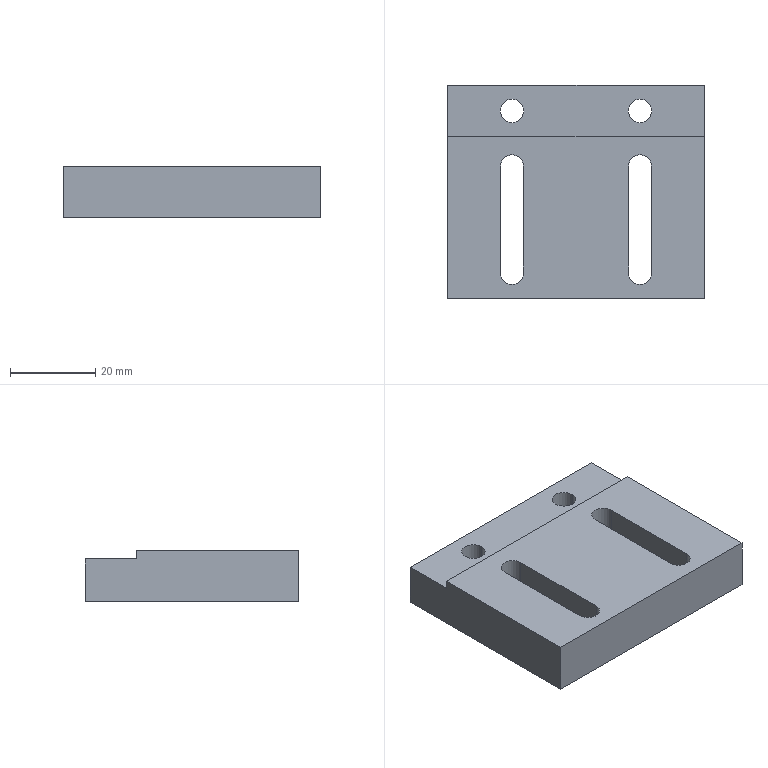Part | SolidWorks | features Cut 1, Extrusion 1, HoleWzd 1, ICE 1 | 1 solid | 26 faces | box 60 x 50 x 12 mm | volume 29704 mm3 | plane 14 | cylinder 12 | commonest cylinder face diameters 5.4 x4 5.5 x4 10 x4
STEP:
#1=CARTESIAN_POINT('',(20.,19.,-0.6));
#2=VERTEX_POINT('',#1);
#3=CARTESIAN_POINT('',(10.,19.,-0.6));
#4=VERTEX_POINT('',#3);
#5=CARTESIAN_POINT('',(15.,19.,-0.6));
#6=DIRECTION('',(0.,0.,-1.));
#7=DIRECTION('',(-1.,0.,0.));
#8=AXIS2_PLACEMENT_3D('',#5,#6,#7);
#9=CIRCLE('',#8,5.);
#10=EDGE_CURVE('',#2,#4,#9,.T.);
#11=ORIENTED_EDGE('',*,*,#10,.F.);
#12=CARTESIAN_POINT('',(20.,19.,-6.));
#13=VERTEX_POINT('',#12);
#14=CARTESIAN_POINT('',(20.,19.,-6.));
#15=DIRECTION('',(0.,0.,-1.));
#16=VECTOR('',#15,1000.);
#17=LINE('',#14,#16);
#18=EDGE_CURVE('',#2,#13,#17,.T.);
#19=ORIENTED_EDGE('',*,*,#18,.T.);
#20=CARTESIAN_POINT('',(10.,19.,-6.));
#21=VERTEX_POINT('',#20);
#22=CARTESIAN_POINT('',(15.,19.,-6.));
#23=DIRECTION('',(0.,0.,-1.));
#24=DIRECTION('',(-1.,0.,0.));
#25=AXIS2_PLACEMENT_3D('',#22,#23,#24);
#26=CIRCLE('',#25,5.);
#27=EDGE_CURVE('',#13,#21,#26,.T.);
#28=ORIENTED_EDGE('',*,*,#27,.T.);
#29=CARTESIAN_POINT('',(10.,19.,-6.));
#30=DIRECTION('',(0.,0.,-1.));
#31=VECTOR('',#30,1000.);
#32=LINE('',#29,#31);
#33=EDGE_CURVE('',#4,#21,#32,.T.);
#34=ORIENTED_EDGE('',*,*,#33,.F.);
#35=EDGE_LOOP('',(#11,#19,#28,#34));
#36=FACE_OUTER_BOUND('',#35,.T.);
#37=CARTESIAN_POINT('',(15.,19.,-6.));
#38=DIRECTION('',(0.,0.,-1.));
#39=DIRECTION('',(-1.,0.,0.));
#40=AXIS2_PLACEMENT_3D('',#37,#38,#39);
#41=CYLINDRICAL_SURFACE('',#40,5.);
#42=ADVANCED_FACE('',(#36),#41,.F.);
#43=CARTESIAN_POINT('',(12.25,19.,4.));
#44=VERTEX_POINT('',#43);
#45=CARTESIAN_POINT('',(17.75,19.,4.));
#46=VERTEX_POINT('',#45);
#47=CARTESIAN_POINT('',(15.,19.,4.));
#48=DIRECTION('',(0.,0.,1.));
#49=DIRECTION('',(1.,0.,0.));
#50=AXIS2_PLACEMENT_3D('',#47,#48,#49);
#51=CIRCLE('',#50,2.75);
#52=EDGE_CURVE('',#44,#46,#51,.T.);
#53=ORIENTED_EDGE('',*,*,#52,.T.);
#54=CARTESIAN_POINT('',(17.75,19.,-0.6));
#55=VERTEX_POINT('',#54);
#56=CARTESIAN_POINT('',(17.75,19.,-6.));
#57=DIRECTION('',(0.,0.,-1.));
#58=VECTOR('',#57,1000.);
#59=LINE('',#56,#58);
#60=EDGE_CURVE('',#46,#55,#59,.T.);
#61=ORIENTED_EDGE('',*,*,#60,.T.);
#62=CARTESIAN_POINT('',(12.25,19.,-0.6));
#63=VERTEX_POINT('',#62);
#64=CARTESIAN_POINT('',(15.,19.,-0.6));
#65=DIRECTION('',(0.,0.,-1.));
#66=DIRECTION('',(-1.,0.,0.));
#67=AXIS2_PLACEMENT_3D('',#64,#65,#66);
#68=CIRCLE('',#67,2.75);
#69=EDGE_CURVE('',#55,#63,#68,.T.);
#70=ORIENTED_EDGE('',*,*,#69,.T.);
#71=CARTESIAN_POINT('',(12.25,19.,-6.));
#72=DIRECTION('',(0.,0.,-1.));
#73=VECTOR('',#72,1000.);
#74=LINE('',#71,#73);
#75=EDGE_CURVE('',#44,#63,#74,.T.);
#76=ORIENTED_EDGE('',*,*,#75,.F.);
#77=EDGE_LOOP('',(#53,#61,#70,#76));
#78=FACE_OUTER_BOUND('',#77,.T.);
#79=CARTESIAN_POINT('',(15.,19.,-6.));
#80=DIRECTION('',(0.,0.,-1.));
#81=DIRECTION('',(-1.,0.,0.));
#82=AXIS2_PLACEMENT_3D('',#79,#80,#81);
#83=CYLINDRICAL_SURFACE('',#82,2.75);
#84=ADVANCED_FACE('',(#78),#83,.F.);
#85=CARTESIAN_POINT('',(-10.,19.,-0.6));
#86=VERTEX_POINT('',#85);
#87=CARTESIAN_POINT('',(-20.,19.,-0.6));
#88=VERTEX_POINT('',#87);
#89=CARTESIAN_POINT('',(-15.,19.,-0.6));
#90=DIRECTION('',(0.,0.,-1.));
#91=DIRECTION('',(-1.,0.,0.));
#92=AXIS2_PLACEMENT_3D('',#89,#90,#91);
#93=CIRCLE('',#92,5.);
#94=EDGE_CURVE('',#86,#88,#93,.T.);
#95=ORIENTED_EDGE('',*,*,#94,.F.);
#96=CARTESIAN_POINT('',(-10.,19.,-6.));
#97=VERTEX_POINT('',#96);
#98=CARTESIAN_POINT('',(-10.,19.,-6.));
#99=DIRECTION('',(0.,0.,-1.));
#100=VECTOR('',#99,1000.);
#101=LINE('',#98,#100);
#102=EDGE_CURVE('',#86,#97,#101,.T.);
#103=ORIENTED_EDGE('',*,*,#102,.T.);
#104=CARTESIAN_POINT('',(-20.,19.,-6.));
#105=VERTEX_POINT('',#104);
#106=CARTESIAN_POINT('',(-15.,19.,-6.));
#107=DIRECTION('',(0.,0.,-1.));
#108=DIRECTION('',(-1.,0.,0.));
#109=AXIS2_PLACEMENT_3D('',#106,#107,#108);
#110=CIRCLE('',#109,5.);
#111=EDGE_CURVE('',#97,#105,#110,.T.);
#112=ORIENTED_EDGE('',*,*,#111,.T.);
#113=CARTESIAN_POINT('',(-20.,19.,-6.));
#114=DIRECTION('',(0.,0.,-1.));
#115=VECTOR('',#114,1000.);
#116=LINE('',#113,#115);
#117=EDGE_CURVE('',#88,#105,#116,.T.);
#118=ORIENTED_EDGE('',*,*,#117,.F.);
#119=EDGE_LOOP('',(#95,#103,#112,#118));
#120=FACE_OUTER_BOUND('',#119,.T.);
#121=CARTESIAN_POINT('',(-15.,19.,-6.));
#122=DIRECTION('',(0.,0.,-1.));
#123=DIRECTION('',(-1.,0.,0.));
#124=AXIS2_PLACEMENT_3D('',#121,#122,#123);
#125=CYLINDRICAL_SURFACE('',#124,5.);
#126=ADVANCED_FACE('',(#120),#125,.F.);
#127=CARTESIAN_POINT('',(-17.75,19.,4.));
#128=VERTEX_POINT('',#127);
#129=CARTESIAN_POINT('',(-12.25,19.,4.));
#130=VERTEX_POINT('',#129);
#131=CARTESIAN_POINT('',(-15.,19.,4.));
#132=DIRECTION('',(0.,0.,1.));
#133=DIRECTION('',(1.,0.,0.));
#134=AXIS2_PLACEMENT_3D('',#131,#132,#133);
#135=CIRCLE('',#134,2.75);
#136=EDGE_CURVE('',#128,#130,#135,.T.);
#137=ORIENTED_EDGE('',*,*,#136,.T.);
#138=CARTESIAN_POINT('',(-12.25,19.,-0.6));
#139=VERTEX_POINT('',#138);
#140=CARTESIAN_POINT('',(-12.25,19.,-6.));
#141=DIRECTION('',(0.,0.,-1.));
#142=VECTOR('',#141,1000.);
#143=LINE('',#140,#142);
#144=EDGE_CURVE('',#130,#139,#143,.T.);
#145=ORIENTED_EDGE('',*,*,#144,.T.);
#146=CARTESIAN_POINT('',(-17.75,19.,-0.6));
#147=VERTEX_POINT('',#146);
#148=CARTESIAN_POINT('',(-15.,19.,-0.6));
#149=DIRECTION('',(0.,0.,-1.));
#150=DIRECTION('',(-1.,0.,0.));
#151=AXIS2_PLACEMENT_3D('',#148,#149,#150);
#152=CIRCLE('',#151,2.75);
#153=EDGE_CURVE('',#139,#147,#152,.T.);
#154=ORIENTED_EDGE('',*,*,#153,.T.);
#155=CARTESIAN_POINT('',(-17.75,19.,-6.));
#156=DIRECTION('',(0.,0.,-1.));
#157=VECTOR('',#156,1000.);
#158=LINE('',#155,#157);
#159=EDGE_CURVE('',#128,#147,#158,.T.);
#160=ORIENTED_EDGE('',*,*,#159,.F.);
#161=EDGE_LOOP('',(#137,#145,#154,#160));
#162=FACE_OUTER_BOUND('',#161,.T.);
#163=CARTESIAN_POINT('',(-15.,19.,-6.));
#164=DIRECTION('',(0.,0.,-1.));
#165=DIRECTION('',(-1.,0.,0.));
#166=AXIS2_PLACEMENT_3D('',#163,#164,#165);
#167=CYLINDRICAL_SURFACE('',#166,2.75);
#168=ADVANCED_FACE('',(#162),#167,.F.);
#169=CARTESIAN_POINT('',(30.,25.,4.));
#170=VERTEX_POINT('',#169);
#171=CARTESIAN_POINT('',(-30.,25.,4.));
#172=VERTEX_POINT('',#171);
#173=CARTESIAN_POINT('',(-30.,25.,4.));
#174=DIRECTION('',(-1.,0.,0.));
#175=VECTOR('',#174,1000.);
#176=LINE('',#173,#175);
#177=EDGE_CURVE('',#170,#172,#176,.T.);
#178=ORIENTED_EDGE('',*,*,#177,.F.);
#179=CARTESIAN_POINT('',(30.,25.,-6.));
#180=VERTEX_POINT('',#179);
#181=CARTESIAN_POINT('',(30.,25.,6.));
#182=DIRECTION('',(0.,0.,-1.));
#183=VECTOR('',#182,1000.);
#184=LINE('',#181,#183);
#185=EDGE_CURVE('',#170,#180,#184,.T.);
#186=ORIENTED_EDGE('',*,*,#185,.T.);
#187=CARTESIAN_POINT('',(-30.,25.,-6.));
#188=VERTEX_POINT('',#187);
#189=CARTESIAN_POINT('',(-30.,25.,-6.));
#190=DIRECTION('',(-1.,0.,0.));
#191=VECTOR('',#190,1000.);
#192=LINE('',#189,#191);
#193=EDGE_CURVE('',#180,#188,#192,.T.);
#194=ORIENTED_EDGE('',*,*,#193,.T.);
#195=CARTESIAN_POINT('',(-30.,25.,6.));
#196=DIRECTION('',(0.,0.,-1.));
#197=VECTOR('',#196,1000.);
#198=LINE('',#195,#197);
#199=EDGE_CURVE('',#172,#188,#198,.T.);
#200=ORIENTED_EDGE('',*,*,#199,.F.);
#201=EDGE_LOOP('',(#178,#186,#194,#200));
#202=FACE_OUTER_BOUND('',#201,.T.);
#203=CARTESIAN_POINT('',(-30.,25.,6.));
#204=DIRECTION('',(0.,-1.,0.));
#205=DIRECTION('',(0.,0.,-1.));
#206=AXIS2_PLACEMENT_3D('',#203,#204,#205);
#207=PLANE('',#206);
#208=ADVANCED_FACE('',(#202),#207,.F.);
#209=CARTESIAN_POINT('',(30.,13.,4.));
#210=VERTEX_POINT('',#209);
#211=CARTESIAN_POINT('',(30.,25.,4.));
#212=DIRECTION('',(0.,1.,0.));
#213=VECTOR('',#212,1000.);
#214=LINE('',#211,#213);
#215=EDGE_CURVE('',#210,#170,#214,.T.);
#216=ORIENTED_EDGE('',*,*,#215,.F.);
#217=CARTESIAN_POINT('',(30.,13.,6.));
#218=VERTEX_POINT('',#217);
#219=CARTESIAN_POINT('',(30.,13.,4.));
#220=DIRECTION('',(0.,0.,1.));
#221=VECTOR('',#220,1000.);
#222=LINE('',#219,#221);
#223=EDGE_CURVE('',#210,#218,#222,.T.);
#224=ORIENTED_EDGE('',*,*,#223,.T.);
#225=CARTESIAN_POINT('',(30.,-25.,6.));
#226=VERTEX_POINT('',#225);
#227=CARTESIAN_POINT('',(30.,25.,6.));
#228=DIRECTION('',(0.,1.,0.));
#229=VECTOR('',#228,1000.);
#230=LINE('',#227,#229);
#231=EDGE_CURVE('',#226,#218,#230,.T.);
#232=ORIENTED_EDGE('',*,*,#231,.F.);
#233=CARTESIAN_POINT('',(30.,-25.,-6.));
#234=VERTEX_POINT('',#233);
#235=CARTESIAN_POINT('',(30.,-25.,6.));
#236=DIRECTION('',(0.,0.,-1.));
#237=VECTOR('',#236,1000.);
#238=LINE('',#235,#237);
#239=EDGE_CURVE('',#226,#234,#238,.T.);
#240=ORIENTED_EDGE('',*,*,#239,.T.);
#241=CARTESIAN_POINT('',(30.,25.,-6.));
#242=DIRECTION('',(0.,1.,0.));
#243=VECTOR('',#242,1000.);
#244=LINE('',#241,#243);
#245=EDGE_CURVE('',#234,#180,#244,.T.);
#246=ORIENTED_EDGE('',*,*,#245,.T.);
#247=ORIENTED_EDGE('',*,*,#185,.F.);
#248=EDGE_LOOP('',(#216,#224,#232,#240,#246,#247));
#249=FACE_OUTER_BOUND('',#248,.T.);
#250=CARTESIAN_POINT('',(30.,25.,6.));
#251=DIRECTION('',(-1.,0.,0.));
#252=DIRECTION('',(0.,-1.,0.));
#253=AXIS2_PLACEMENT_3D('',#250,#251,#252);
#254=PLANE('',#253);
#255=ADVANCED_FACE('',(#249),#254,.F.);
#256=CARTESIAN_POINT('',(-30.,13.,6.));
#257=VERTEX_POINT('',#256);
#258=CARTESIAN_POINT('',(-30.,-25.,6.));
#259=VERTEX_POINT('',#258);
#260=CARTESIAN_POINT('',(-30.,25.,6.));
#261=DIRECTION('',(0.,-1.,0.));
#262=VECTOR('',#261,1000.);
#263=LINE('',#260,#262);
#264=EDGE_CURVE('',#257,#259,#263,.T.);
#265=ORIENTED_EDGE('',*,*,#264,.F.);
#266=CARTESIAN_POINT('',(-30.,13.,4.));
#267=VERTEX_POINT('',#266);
#268=CARTESIAN_POINT('',(-30.,13.,4.));
#269=DIRECTION('',(0.,0.,1.));
#270=VECTOR('',#269,1000.);
#271=LINE('',#268,#270);
#272=EDGE_CURVE('',#267,#257,#271,.T.);
#273=ORIENTED_EDGE('',*,*,#272,.F.);
#274=CARTESIAN_POINT('',(-30.,25.,4.));
#275=DIRECTION('',(0.,-1.,0.));
#276=VECTOR('',#275,1000.);
#277=LINE('',#274,#276);
#278=EDGE_CURVE('',#172,#267,#277,.T.);
#279=ORIENTED_EDGE('',*,*,#278,.F.);
#280=ORIENTED_EDGE('',*,*,#199,.T.);
#281=CARTESIAN_POINT('',(-30.,-25.,-6.));
#282=VERTEX_POINT('',#281);
#283=CARTESIAN_POINT('',(-30.,25.,-6.));
#284=DIRECTION('',(0.,-1.,0.));
#285=VECTOR('',#284,1000.);
#286=LINE('',#283,#285);
#287=EDGE_CURVE('',#188,#282,#286,.T.);
#288=ORIENTED_EDGE('',*,*,#287,.T.);
#289=CARTESIAN_POINT('',(-30.,-25.,6.));
#290=DIRECTION('',(0.,0.,-1.));
#291=VECTOR('',#290,1000.);
#292=LINE('',#289,#291);
#293=EDGE_CURVE('',#259,#282,#292,.T.);
#294=ORIENTED_EDGE('',*,*,#293,.F.);
#295=EDGE_LOOP('',(#265,#273,#279,#280,#288,#294));
#296=FACE_OUTER_BOUND('',#295,.T.);
#297=CARTESIAN_POINT('',(-30.,25.,6.));
#298=DIRECTION('',(1.,0.,0.));
#299=DIRECTION('',(0.,1.,0.));
#300=AXIS2_PLACEMENT_3D('',#297,#298,#299);
#301=PLANE('',#300);
#302=ADVANCED_FACE('',(#296),#301,.F.);
#303=CARTESIAN_POINT('',(-30.,-25.,-6.));
#304=DIRECTION('',(1.,0.,0.));
#305=VECTOR('',#304,1000.);
#306=LINE('',#303,#305);
#307=EDGE_CURVE('',#282,#234,#306,.T.);
#308=ORIENTED_EDGE('',*,*,#307,.T.);
#309=ORIENTED_EDGE('',*,*,#239,.F.);
#310=CARTESIAN_POINT('',(-30.,-25.,6.));
#311=DIRECTION('',(1.,0.,0.));
#312=VECTOR('',#311,1000.);
#313=LINE('',#310,#312);
#314=EDGE_CURVE('',#259,#226,#313,.T.);
#315=ORIENTED_EDGE('',*,*,#314,.F.);
#316=ORIENTED_EDGE('',*,*,#293,.T.);
#317=EDGE_LOOP('',(#308,#309,#315,#316));
#318=FACE_OUTER_BOUND('',#317,.T.);
#319=CARTESIAN_POINT('',(-30.,-25.,6.));
#320=DIRECTION('',(0.,1.,0.));
#321=DIRECTION('',(0.,0.,1.));
#322=AXIS2_PLACEMENT_3D('',#319,#320,#321);
#323=PLANE('',#322);
#324=ADVANCED_FACE('',(#318),#323,.F.);
#325=CARTESIAN_POINT('',(-17.7,-19.,6.));
#326=VERTEX_POINT('',#325);
#327=CARTESIAN_POINT('',(-12.3,-19.,6.));
#328=VERTEX_POINT('',#327);
#329=CARTESIAN_POINT('',(-15.,-19.,6.));
#330=DIRECTION('',(0.,0.,1.));
#331=DIRECTION('',(1.,0.,0.));
#332=AXIS2_PLACEMENT_3D('',#329,#330,#331);
#333=CIRCLE('',#332,2.7);
#334=EDGE_CURVE('',#326,#328,#333,.T.);
#335=ORIENTED_EDGE('',*,*,#334,.F.);
#336=CARTESIAN_POINT('',(-17.7,6.,6.));
#337=VERTEX_POINT('',#336);
#338=CARTESIAN_POINT('',(-17.7,-19.,6.));
#339=DIRECTION('',(0.,-1.,0.));
#340=VECTOR('',#339,1000.);
#341=LINE('',#338,#340);
#342=EDGE_CURVE('',#337,#326,#341,.T.);
#343=ORIENTED_EDGE('',*,*,#342,.F.);
#344=CARTESIAN_POINT('',(-12.3,6.,6.));
#345=VERTEX_POINT('',#344);
#346=CARTESIAN_POINT('',(-15.,6.,6.));
#347=DIRECTION('',(0.,0.,1.));
#348=DIRECTION('',(1.,0.,0.));
#349=AXIS2_PLACEMENT_3D('',#346,#347,#348);
#350=CIRCLE('',#349,2.7);
#351=EDGE_CURVE('',#345,#337,#350,.T.);
#352=ORIENTED_EDGE('',*,*,#351,.F.);
#353=CARTESIAN_POINT('',(-12.3,-19.,6.));
#354=DIRECTION('',(0.,1.,0.));
#355=VECTOR('',#354,1000.);
#356=LINE('',#353,#355);
#357=EDGE_CURVE('',#328,#345,#356,.T.);
#358=ORIENTED_EDGE('',*,*,#357,.F.);
#359=EDGE_LOOP('',(#335,#343,#352,#358));
#360=FACE_BOUND('',#359,.T.);
#361=CARTESIAN_POINT('',(12.3,-19.,6.));
#362=VERTEX_POINT('',#361);
#363=CARTESIAN_POINT('',(17.7,-19.,6.));
#364=VERTEX_POINT('',#363);
#365=CARTESIAN_POINT('',(15.,-19.,6.));
#366=DIRECTION('',(0.,0.,1.));
#367=DIRECTION('',(1.,0.,0.));
#368=AXIS2_PLACEMENT_3D('',#365,#366,#367);
#369=CIRCLE('',#368,2.7);
#370=EDGE_CURVE('',#362,#364,#369,.T.);
#371=ORIENTED_EDGE('',*,*,#370,.F.);
#372=CARTESIAN_POINT('',(12.3,6.,6.));
#373=VERTEX_POINT('',#372);
#374=CARTESIAN_POINT('',(12.3,-19.,6.));
#375=DIRECTION('',(0.,-1.,0.));
#376=VECTOR('',#375,1000.);
#377=LINE('',#374,#376);
#378=EDGE_CURVE('',#373,#362,#377,.T.);
#379=ORIENTED_EDGE('',*,*,#378,.F.);
#380=CARTESIAN_POINT('',(17.7,6.,6.));
#381=VERTEX_POINT('',#380);
#382=CARTESIAN_POINT('',(15.,6.,6.));
#383=DIRECTION('',(0.,0.,1.));
#384=DIRECTION('',(1.,0.,0.));
#385=AXIS2_PLACEMENT_3D('',#382,#383,#384);
#386=CIRCLE('',#385,2.7);
#387=EDGE_CURVE('',#381,#373,#386,.T.);
#388=ORIENTED_EDGE('',*,*,#387,.F.);
#389=CARTESIAN_POINT('',(17.7,-19.,6.));
#390=DIRECTION('',(0.,1.,0.));
#391=VECTOR('',#390,1000.);
#392=LINE('',#389,#391);
#393=EDGE_CURVE('',#364,#381,#392,.T.);
#394=ORIENTED_EDGE('',*,*,#393,.F.);
#395=EDGE_LOOP('',(#371,#379,#388,#394));
#396=FACE_BOUND('',#395,.T.);
#397=CARTESIAN_POINT('',(-30.,13.,6.));
#398=DIRECTION('',(1.,0.,0.));
#399=VECTOR('',#398,1000.);
#400=LINE('',#397,#399);
#401=EDGE_CURVE('',#257,#218,#400,.T.);
#402=ORIENTED_EDGE('',*,*,#401,.F.);
#403=ORIENTED_EDGE('',*,*,#264,.T.);
#404=ORIENTED_EDGE('',*,*,#314,.T.);
#405=ORIENTED_EDGE('',*,*,#231,.T.);
#406=EDGE_LOOP('',(#402,#403,#404,#405));
#407=FACE_OUTER_BOUND('',#406,.T.);
#408=CARTESIAN_POINT('',(0.,0.,6.));
#409=DIRECTION('',(0.,0.,1.));
#410=DIRECTION('',(1.,0.,0.));
#411=AXIS2_PLACEMENT_3D('',#408,#409,#410);
#412=PLANE('',#411);
#413=ADVANCED_FACE('',(#360,#396,#407),#412,.T.);
#414=CARTESIAN_POINT('',(15.,19.,-6.));
#415=DIRECTION('',(0.,0.,-1.));
#416=DIRECTION('',(-1.,0.,0.));
#417=AXIS2_PLACEMENT_3D('',#414,#415,#416);
#418=CIRCLE('',#417,5.);
#419=EDGE_CURVE('',#21,#13,#418,.T.);
#420=ORIENTED_EDGE('',*,*,#419,.F.);
#421=ORIENTED_EDGE('',*,*,#27,.F.);
#422=EDGE_LOOP('',(#420,#421));
#423=FACE_BOUND('',#422,.T.);
#424=CARTESIAN_POINT('',(-15.,19.,-6.));
#425=DIRECTION('',(0.,0.,-1.));
#426=DIRECTION('',(-1.,0.,0.));
#427=AXIS2_PLACEMENT_3D('',#424,#425,#426);
#428=CIRCLE('',#427,5.);
#429=EDGE_CURVE('',#105,#97,#428,.T.);
#430=ORIENTED_EDGE('',*,*,#429,.F.);
#431=ORIENTED_EDGE('',*,*,#111,.F.);
#432=EDGE_LOOP('',(#430,#431));
#433=FACE_BOUND('',#432,.T.);
#434=CARTESIAN_POINT('',(-17.7,6.,-6.));
#435=VERTEX_POINT('',#434);
#436=CARTESIAN_POINT('',(-17.7,-19.,-6.));
#437=VERTEX_POINT('',#436);
#438=CARTESIAN_POINT('',(-17.7,-19.,-6.));
#439=DIRECTION('',(0.,-1.,0.));
#440=VECTOR('',#439,1000.);
#441=LINE('',#438,#440);
#442=EDGE_CURVE('',#435,#437,#441,.T.);
#443=ORIENTED_EDGE('',*,*,#442,.T.);
#444=CARTESIAN_POINT('',(-12.3,-19.,-6.));
#445=VERTEX_POINT('',#444);
#446=CARTESIAN_POINT('',(-15.,-19.,-6.));
#447=DIRECTION('',(0.,0.,1.));
#448=DIRECTION('',(1.,0.,0.));
#449=AXIS2_PLACEMENT_3D('',#446,#447,#448);
#450=CIRCLE('',#449,2.7);
#451=EDGE_CURVE('',#437,#445,#450,.T.);
#452=ORIENTED_EDGE('',*,*,#451,.T.);
#453=CARTESIAN_POINT('',(-12.3,6.,-6.));
#454=VERTEX_POINT('',#453);
#455=CARTESIAN_POINT('',(-12.3,-19.,-6.));
#456=DIRECTION('',(0.,1.,0.));
#457=VECTOR('',#456,1000.);
#458=LINE('',#455,#457);
#459=EDGE_CURVE('',#445,#454,#458,.T.);
#460=ORIENTED_EDGE('',*,*,#459,.T.);
#461=CARTESIAN_POINT('',(-15.,6.,-6.));
#462=DIRECTION('',(0.,0.,1.));
#463=DIRECTION('',(1.,0.,0.));
#464=AXIS2_PLACEMENT_3D('',#461,#462,#463);
#465=CIRCLE('',#464,2.7);
#466=EDGE_CURVE('',#454,#435,#465,.T.);
#467=ORIENTED_EDGE('',*,*,#466,.T.);
#468=EDGE_LOOP('',(#443,#452,#460,#467));
#469=FACE_BOUND('',#468,.T.);
#470=CARTESIAN_POINT('',(12.3,6.,-6.));
#471=VERTEX_POINT('',#470);
#472=CARTESIAN_POINT('',(12.3,-19.,-6.));
#473=VERTEX_POINT('',#472);
#474=CARTESIAN_POINT('',(12.3,-19.,-6.));
#475=DIRECTION('',(0.,-1.,0.));
#476=VECTOR('',#475,1000.);
#477=LINE('',#474,#476);
#478=EDGE_CURVE('',#471,#473,#477,.T.);
#479=ORIENTED_EDGE('',*,*,#478,.T.);
#480=CARTESIAN_POINT('',(17.7,-19.,-6.));
#481=VERTEX_POINT('',#480);
#482=CARTESIAN_POINT('',(15.,-19.,-6.));
#483=DIRECTION('',(0.,0.,1.));
#484=DIRECTION('',(1.,0.,0.));
#485=AXIS2_PLACEMENT_3D('',#482,#483,#484);
#486=CIRCLE('',#485,2.7);
#487=EDGE_CURVE('',#473,#481,#486,.T.);
#488=ORIENTED_EDGE('',*,*,#487,.T.);
#489=CARTESIAN_POINT('',(17.7,6.,-6.));
#490=VERTEX_POINT('',#489);
#491=CARTESIAN_POINT('',(17.7,-19.,-6.));
#492=DIRECTION('',(0.,1.,0.));
#493=VECTOR('',#492,1000.);
#494=LINE('',#491,#493);
#495=EDGE_CURVE('',#481,#490,#494,.T.);
#496=ORIENTED_EDGE('',*,*,#495,.T.);
#497=CARTESIAN_POINT('',(15.,6.,-6.));
#498=DIRECTION('',(0.,0.,1.));
#499=DIRECTION('',(1.,0.,0.));
#500=AXIS2_PLACEMENT_3D('',#497,#498,#499);
#501=CIRCLE('',#500,2.7);
#502=EDGE_CURVE('',#490,#471,#501,.T.);
#503=ORIENTED_EDGE('',*,*,#502,.T.);
#504=EDGE_LOOP('',(#479,#488,#496,#503));
#505=FACE_BOUND('',#504,.T.);
#506=ORIENTED_EDGE('',*,*,#245,.F.);
#507=ORIENTED_EDGE('',*,*,#307,.F.);
#508=ORIENTED_EDGE('',*,*,#287,.F.);
#509=ORIENTED_EDGE('',*,*,#193,.F.);
#510=EDGE_LOOP('',(#506,#507,#508,#509));
#511=FACE_OUTER_BOUND('',#510,.T.);
#512=CARTESIAN_POINT('',(0.,0.,-6.));
#513=DIRECTION('',(0.,0.,1.));
#514=DIRECTION('',(1.,0.,0.));
#515=AXIS2_PLACEMENT_3D('',#512,#513,#514);
#516=PLANE('',#515);
#517=ADVANCED_FACE('',(#423,#433,#469,#505,#511),#516,.F.);
#518=ORIENTED_EDGE('',*,*,#401,.T.);
#519=ORIENTED_EDGE('',*,*,#223,.F.);
#520=CARTESIAN_POINT('',(-30.,13.,4.));
#521=DIRECTION('',(1.,0.,0.));
#522=VECTOR('',#521,1000.);
#523=LINE('',#520,#522);
#524=EDGE_CURVE('',#267,#210,#523,.T.);
#525=ORIENTED_EDGE('',*,*,#524,.F.);
#526=ORIENTED_EDGE('',*,*,#272,.T.);
#527=EDGE_LOOP('',(#518,#519,#525,#526));
#528=FACE_OUTER_BOUND('',#527,.T.);
#529=CARTESIAN_POINT('',(-30.,13.,4.));
#530=DIRECTION('',(0.,-1.,0.));
#531=DIRECTION('',(0.,0.,-1.));
#532=AXIS2_PLACEMENT_3D('',#529,#530,#531);
#533=PLANE('',#532);
#534=ADVANCED_FACE('',(#528),#533,.F.);
#535=ORIENTED_EDGE('',*,*,#52,.F.);
#536=CARTESIAN_POINT('',(15.,19.,4.));
#537=DIRECTION('',(0.,0.,1.));
#538=DIRECTION('',(1.,0.,0.));
#539=AXIS2_PLACEMENT_3D('',#536,#537,#538);
#540=CIRCLE('',#539,2.75);
#541=EDGE_CURVE('',#46,#44,#540,.T.);
#542=ORIENTED_EDGE('',*,*,#541,.F.);
#543=EDGE_LOOP('',(#535,#542));
#544=FACE_BOUND('',#543,.T.);
#545=ORIENTED_EDGE('',*,*,#136,.F.);
#546=CARTESIAN_POINT('',(-15.,19.,4.));
#547=DIRECTION('',(0.,0.,1.));
#548=DIRECTION('',(1.,0.,0.));
#549=AXIS2_PLACEMENT_3D('',#546,#547,#548);
#550=CIRCLE('',#549,2.75);
#551=EDGE_CURVE('',#130,#128,#550,.T.);
#552=ORIENTED_EDGE('',*,*,#551,.F.);
#553=EDGE_LOOP('',(#545,#552));
#554=FACE_BOUND('',#553,.T.);
#555=ORIENTED_EDGE('',*,*,#278,.T.);
#556=ORIENTED_EDGE('',*,*,#524,.T.);
#557=ORIENTED_EDGE('',*,*,#215,.T.);
#558=ORIENTED_EDGE('',*,*,#177,.T.);
#559=EDGE_LOOP('',(#555,#556,#557,#558));
#560=FACE_OUTER_BOUND('',#559,.T.);
#561=CARTESIAN_POINT('',(0.,0.,4.));
#562=DIRECTION('',(0.,0.,1.));
#563=DIRECTION('',(1.,0.,0.));
#564=AXIS2_PLACEMENT_3D('',#561,#562,#563);
#565=PLANE('',#564);
#566=ADVANCED_FACE('',(#544,#554,#560),#565,.T.);
#567=ORIENTED_EDGE('',*,*,#370,.T.);
#568=CARTESIAN_POINT('',(17.7,-19.,-6.));
#569=DIRECTION('',(0.,0.,1.));
#570=VECTOR('',#569,1000.);
#571=LINE('',#568,#570);
#572=EDGE_CURVE('',#481,#364,#571,.T.);
#573=ORIENTED_EDGE('',*,*,#572,.F.);
#574=ORIENTED_EDGE('',*,*,#487,.F.);
#575=CARTESIAN_POINT('',(12.3,-19.,-6.));
#576=DIRECTION('',(0.,0.,1.));
#577=VECTOR('',#576,1000.);
#578=LINE('',#575,#577);
#579=EDGE_CURVE('',#473,#362,#578,.T.);
#580=ORIENTED_EDGE('',*,*,#579,.T.);
#581=EDGE_LOOP('',(#567,#573,#574,#580));
#582=FACE_OUTER_BOUND('',#581,.T.);
#583=CARTESIAN_POINT('',(15.,-19.,-6.));
#584=DIRECTION('',(0.,0.,1.));
#585=DIRECTION('',(1.,0.,0.));
#586=AXIS2_PLACEMENT_3D('',#583,#584,#585);
#587=CYLINDRICAL_SURFACE('',#586,2.7);
#588=ADVANCED_FACE('',(#582),#587,.F.);
#589=ORIENTED_EDGE('',*,*,#378,.T.);
#590=ORIENTED_EDGE('',*,*,#579,.F.);
#591=ORIENTED_EDGE('',*,*,#478,.F.);
#592=CARTESIAN_POINT('',(12.3,6.,-6.));
#593=DIRECTION('',(0.,0.,1.));
#594=VECTOR('',#593,1000.);
#595=LINE('',#592,#594);
#596=EDGE_CURVE('',#471,#373,#595,.T.);
#597=ORIENTED_EDGE('',*,*,#596,.T.);
#598=EDGE_LOOP('',(#589,#590,#591,#597));
#599=FACE_OUTER_BOUND('',#598,.T.);
#600=CARTESIAN_POINT('',(12.3,-19.,-6.));
#601=DIRECTION('',(-1.,0.,0.));
#602=DIRECTION('',(0.,-1.,0.));
#603=AXIS2_PLACEMENT_3D('',#600,#601,#602);
#604=PLANE('',#603);
#605=ADVANCED_FACE('',(#599),#604,.F.);
#606=ORIENTED_EDGE('',*,*,#387,.T.);
#607=ORIENTED_EDGE('',*,*,#596,.F.);
#608=ORIENTED_EDGE('',*,*,#502,.F.);
#609=CARTESIAN_POINT('',(17.7,6.,-6.));
#610=DIRECTION('',(0.,0.,1.));
#611=VECTOR('',#610,1000.);
#612=LINE('',#609,#611);
#613=EDGE_CURVE('',#490,#381,#612,.T.);
#614=ORIENTED_EDGE('',*,*,#613,.T.);
#615=EDGE_LOOP('',(#606,#607,#608,#614));
#616=FACE_OUTER_BOUND('',#615,.T.);
#617=CARTESIAN_POINT('',(15.,6.,-6.));
#618=DIRECTION('',(0.,0.,1.));
#619=DIRECTION('',(1.,0.,0.));
#620=AXIS2_PLACEMENT_3D('',#617,#618,#619);
#621=CYLINDRICAL_SURFACE('',#620,2.7);
#622=ADVANCED_FACE('',(#616),#621,.F.);
#623=ORIENTED_EDGE('',*,*,#393,.T.);
#624=ORIENTED_EDGE('',*,*,#613,.F.);
#625=ORIENTED_EDGE('',*,*,#495,.F.);
#626=ORIENTED_EDGE('',*,*,#572,.T.);
#627=EDGE_LOOP('',(#623,#624,#625,#626));
#628=FACE_OUTER_BOUND('',#627,.T.);
#629=CARTESIAN_POINT('',(17.7,-19.,-6.));
#630=DIRECTION('',(1.,0.,0.));
#631=DIRECTION('',(0.,0.,-1.));
#632=AXIS2_PLACEMENT_3D('',#629,#630,#631);
#633=PLANE('',#632);
#634=ADVANCED_FACE('',(#628),#633,.F.);
#635=ORIENTED_EDGE('',*,*,#334,.T.);
#636=CARTESIAN_POINT('',(-12.3,-19.,-6.));
#637=DIRECTION('',(0.,0.,1.));
#638=VECTOR('',#637,1000.);
#639=LINE('',#636,#638);
#640=EDGE_CURVE('',#445,#328,#639,.T.);
#641=ORIENTED_EDGE('',*,*,#640,.F.);
#642=ORIENTED_EDGE('',*,*,#451,.F.);
#643=CARTESIAN_POINT('',(-17.7,-19.,-6.));
#644=DIRECTION('',(0.,0.,1.));
#645=VECTOR('',#644,1000.);
#646=LINE('',#643,#645);
#647=EDGE_CURVE('',#437,#326,#646,.T.);
#648=ORIENTED_EDGE('',*,*,#647,.T.);
#649=EDGE_LOOP('',(#635,#641,#642,#648));
#650=FACE_OUTER_BOUND('',#649,.T.);
#651=CARTESIAN_POINT('',(-15.,-19.,-6.));
#652=DIRECTION('',(0.,0.,1.));
#653=DIRECTION('',(1.,0.,0.));
#654=AXIS2_PLACEMENT_3D('',#651,#652,#653);
#655=CYLINDRICAL_SURFACE('',#654,2.7);
#656=ADVANCED_FACE('',(#650),#655,.F.);
#657=ORIENTED_EDGE('',*,*,#342,.T.);
#658=ORIENTED_EDGE('',*,*,#647,.F.);
#659=ORIENTED_EDGE('',*,*,#442,.F.);
#660=CARTESIAN_POINT('',(-17.7,6.,-6.));
#661=DIRECTION('',(0.,0.,1.));
#662=VECTOR('',#661,1000.);
#663=LINE('',#660,#662);
#664=EDGE_CURVE('',#435,#337,#663,.T.);
#665=ORIENTED_EDGE('',*,*,#664,.T.);
#666=EDGE_LOOP('',(#657,#658,#659,#665));
#667=FACE_OUTER_BOUND('',#666,.T.);
#668=CARTESIAN_POINT('',(-17.7,-19.,-6.));
#669=DIRECTION('',(-1.,0.,0.));
#670=DIRECTION('',(0.,-1.,0.));
#671=AXIS2_PLACEMENT_3D('',#668,#669,#670);
#672=PLANE('',#671);
#673=ADVANCED_FACE('',(#667),#672,.F.);
#674=ORIENTED_EDGE('',*,*,#351,.T.);
#675=ORIENTED_EDGE('',*,*,#664,.F.);
#676=ORIENTED_EDGE('',*,*,#466,.F.);
#677=CARTESIAN_POINT('',(-12.3,6.,-6.));
#678=DIRECTION('',(0.,0.,1.));
#679=VECTOR('',#678,1000.);
#680=LINE('',#677,#679);
#681=EDGE_CURVE('',#454,#345,#680,.T.);
#682=ORIENTED_EDGE('',*,*,#681,.T.);
#683=EDGE_LOOP('',(#674,#675,#676,#682));
#684=FACE_OUTER_BOUND('',#683,.T.);
#685=CARTESIAN_POINT('',(-15.,6.,-6.));
#686=DIRECTION('',(0.,0.,1.));
#687=DIRECTION('',(1.,0.,0.));
#688=AXIS2_PLACEMENT_3D('',#685,#686,#687);
#689=CYLINDRICAL_SURFACE('',#688,2.7);
#690=ADVANCED_FACE('',(#684),#689,.F.);
#691=ORIENTED_EDGE('',*,*,#357,.T.);
#692=ORIENTED_EDGE('',*,*,#681,.F.);
#693=ORIENTED_EDGE('',*,*,#459,.F.);
#694=ORIENTED_EDGE('',*,*,#640,.T.);
#695=EDGE_LOOP('',(#691,#692,#693,#694));
#696=FACE_OUTER_BOUND('',#695,.T.);
#697=CARTESIAN_POINT('',(-12.3,-19.,-6.));
#698=DIRECTION('',(1.,0.,0.));
#699=DIRECTION('',(0.,1.,0.));
#700=AXIS2_PLACEMENT_3D('',#697,#698,#699);
#701=PLANE('',#700);
#702=ADVANCED_FACE('',(#696),#701,.F.);
#703=ORIENTED_EDGE('',*,*,#144,.F.);
#704=ORIENTED_EDGE('',*,*,#551,.T.);
#705=ORIENTED_EDGE('',*,*,#159,.T.);
#706=CARTESIAN_POINT('',(-15.,19.,-0.6));
#707=DIRECTION('',(0.,0.,-1.));
#708=DIRECTION('',(-1.,0.,0.));
#709=AXIS2_PLACEMENT_3D('',#706,#707,#708);
#710=CIRCLE('',#709,2.75);
#711=EDGE_CURVE('',#147,#139,#710,.T.);
#712=ORIENTED_EDGE('',*,*,#711,.T.);
#713=EDGE_LOOP('',(#703,#704,#705,#712));
#714=FACE_OUTER_BOUND('',#713,.T.);
#715=CARTESIAN_POINT('',(-15.,19.,-6.));
#716=DIRECTION('',(0.,0.,-1.));
#717=DIRECTION('',(-1.,0.,0.));
#718=AXIS2_PLACEMENT_3D('',#715,#716,#717);
#719=CYLINDRICAL_SURFACE('',#718,2.75);
#720=ADVANCED_FACE('',(#714),#719,.F.);
#721=ORIENTED_EDGE('',*,*,#711,.F.);
#722=ORIENTED_EDGE('',*,*,#153,.F.);
#723=EDGE_LOOP('',(#721,#722));
#724=FACE_BOUND('',#723,.T.);
#725=CARTESIAN_POINT('',(-15.,19.,-0.6));
#726=DIRECTION('',(0.,0.,-1.));
#727=DIRECTION('',(-1.,0.,0.));
#728=AXIS2_PLACEMENT_3D('',#725,#726,#727);
#729=CIRCLE('',#728,5.);
#730=EDGE_CURVE('',#88,#86,#729,.T.);
#731=ORIENTED_EDGE('',*,*,#730,.T.);
#732=ORIENTED_EDGE('',*,*,#94,.T.);
#733=EDGE_LOOP('',(#731,#732));
#734=FACE_OUTER_BOUND('',#733,.T.);
#735=CARTESIAN_POINT('',(-12.25,19.,-0.6));
#736=DIRECTION('',(0.,0.,1.));
#737=DIRECTION('',(1.,0.,0.));
#738=AXIS2_PLACEMENT_3D('',#735,#736,#737);
#739=PLANE('',#738);
#740=ADVANCED_FACE('',(#724,#734),#739,.F.);
#741=ORIENTED_EDGE('',*,*,#102,.F.);
#742=ORIENTED_EDGE('',*,*,#730,.F.);
#743=ORIENTED_EDGE('',*,*,#117,.T.);
#744=ORIENTED_EDGE('',*,*,#429,.T.);
#745=EDGE_LOOP('',(#741,#742,#743,#744));
#746=FACE_OUTER_BOUND('',#745,.T.);
#747=CARTESIAN_POINT('',(-15.,19.,-6.));
#748=DIRECTION('',(0.,0.,-1.));
#749=DIRECTION('',(-1.,0.,0.));
#750=AXIS2_PLACEMENT_3D('',#747,#748,#749);
#751=CYLINDRICAL_SURFACE('',#750,5.);
#752=ADVANCED_FACE('',(#746),#751,.F.);
#753=ORIENTED_EDGE('',*,*,#60,.F.);
#754=ORIENTED_EDGE('',*,*,#541,.T.);
#755=ORIENTED_EDGE('',*,*,#75,.T.);
#756=CARTESIAN_POINT('',(15.,19.,-0.6));
#757=DIRECTION('',(0.,0.,-1.));
#758=DIRECTION('',(-1.,0.,0.));
#759=AXIS2_PLACEMENT_3D('',#756,#757,#758);
#760=CIRCLE('',#759,2.75);
#761=EDGE_CURVE('',#63,#55,#760,.T.);
#762=ORIENTED_EDGE('',*,*,#761,.T.);
#763=EDGE_LOOP('',(#753,#754,#755,#762));
#764=FACE_OUTER_BOUND('',#763,.T.);
#765=CARTESIAN_POINT('',(15.,19.,-6.));
#766=DIRECTION('',(0.,0.,-1.));
#767=DIRECTION('',(-1.,0.,0.));
#768=AXIS2_PLACEMENT_3D('',#765,#766,#767);
#769=CYLINDRICAL_SURFACE('',#768,2.75);
#770=ADVANCED_FACE('',(#764),#769,.F.);
#771=ORIENTED_EDGE('',*,*,#761,.F.);
#772=ORIENTED_EDGE('',*,*,#69,.F.);
#773=EDGE_LOOP('',(#771,#772));
#774=FACE_BOUND('',#773,.T.);
#775=CARTESIAN_POINT('',(15.,19.,-0.6));
#776=DIRECTION('',(0.,0.,-1.));
#777=DIRECTION('',(-1.,0.,0.));
#778=AXIS2_PLACEMENT_3D('',#775,#776,#777);
#779=CIRCLE('',#778,5.);
#780=EDGE_CURVE('',#4,#2,#779,.T.);
#781=ORIENTED_EDGE('',*,*,#780,.T.);
#782=ORIENTED_EDGE('',*,*,#10,.T.);
#783=EDGE_LOOP('',(#781,#782));
#784=FACE_OUTER_BOUND('',#783,.T.);
#785=CARTESIAN_POINT('',(17.75,19.,-0.6));
#786=DIRECTION('',(0.,0.,1.));
#787=DIRECTION('',(1.,0.,0.));
#788=AXIS2_PLACEMENT_3D('',#785,#786,#787);
#789=PLANE('',#788);
#790=ADVANCED_FACE('',(#774,#784),#789,.F.);
#791=ORIENTED_EDGE('',*,*,#18,.F.);
#792=ORIENTED_EDGE('',*,*,#780,.F.);
#793=ORIENTED_EDGE('',*,*,#33,.T.);
#794=ORIENTED_EDGE('',*,*,#419,.T.);
#795=EDGE_LOOP('',(#791,#792,#793,#794));
#796=FACE_OUTER_BOUND('',#795,.T.);
#797=CARTESIAN_POINT('',(15.,19.,-6.));
#798=DIRECTION('',(0.,0.,-1.));
#799=DIRECTION('',(-1.,0.,0.));
#800=AXIS2_PLACEMENT_3D('',#797,#798,#799);
#801=CYLINDRICAL_SURFACE('',#800,5.);
#802=ADVANCED_FACE('',(#796),#801,.F.);
#803=CLOSED_SHELL('',(#42,#84,#126,#168,#208,#255,#302,#324,#413,#517,#534,#566,#588,#605,#622,#634,#656,#673,#690,#702,#720,#740,#752,#770,#790,#802));
#804=MANIFOLD_SOLID_BREP('',#803);
#805=CARTESIAN_POINT('',(0.,0.,0.));
#806=DIRECTION('',(0.,0.,1.));
#807=DIRECTION('',(1.,0.,0.));
#808=AXIS2_PLACEMENT_3D('',#805,#806,#807);
#809=(LENGTH_UNIT()NAMED_UNIT(*)SI_UNIT(.MILLI.,.METRE.));
#810=UNCERTAINTY_MEASURE_WITH_UNIT(LENGTH_MEASURE(0.00001),#809,'','');
#811=(NAMED_UNIT(*)PLANE_ANGLE_UNIT()SI_UNIT($,.RADIAN.));
#812=(NAMED_UNIT(*)SI_UNIT($,.STERADIAN.)SOLID_ANGLE_UNIT());
#813=(GEOMETRIC_REPRESENTATION_CONTEXT(3)GLOBAL_UNCERTAINTY_ASSIGNED_CONTEXT((#810))GLOBAL_UNIT_ASSIGNED_CONTEXT((#809,#811,#812))REPRESENTATION_CONTEXT('',''));
#814=ADVANCED_BREP_SHAPE_REPRESENTATION('',(#804,#808),#813);